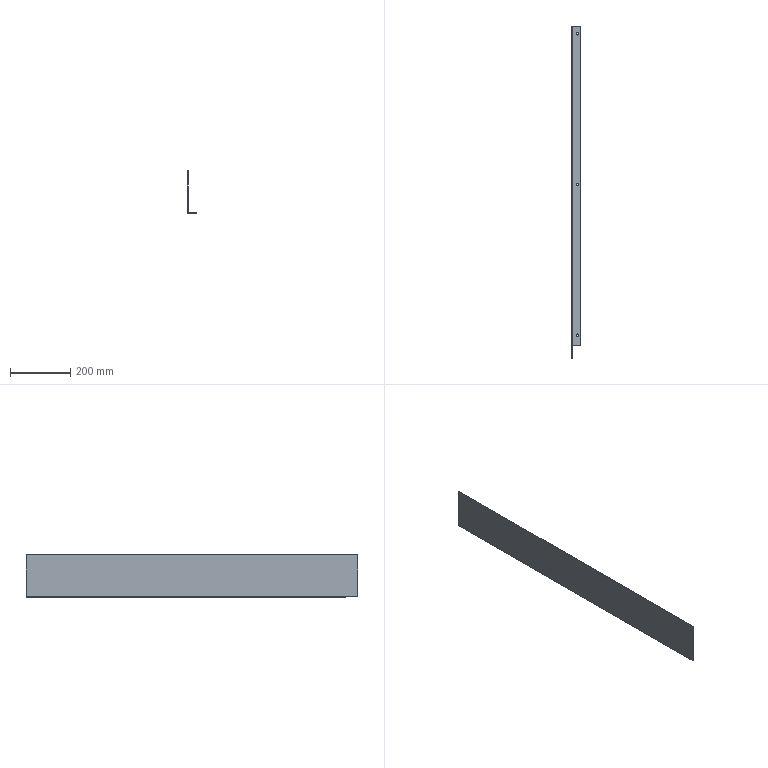Part | STEP file | PN_0008 Partition plate2 | 1 solid | 18 faces | box 30 x 1100 x 140 mm | volume 365122 mm3 | plane 10 | cone 6 | cylinder 2 | commonest cylinder face diameters 2 x1 6 x1
STEP:
#1=CARTESIAN_POINT('',(0.,0.,0.));
#2=DIRECTION('',(0.,0.,1.));
#3=DIRECTION('',(1.,0.,0.));
#4=AXIS2_PLACEMENT_3D('',#1,#2,#3);
#5=CARTESIAN_POINT('',(22.7,525.,0.));
#6=VERTEX_POINT('',#5);
#7=CARTESIAN_POINT('',(24.7,525.,2.));
#8=VERTEX_POINT('',#7);
#9=CARTESIAN_POINT('',(24.7,525.,2.));
#10=DIRECTION('',(0.7071,0.,0.7071));
#11=VECTOR('',#10,1.);
#12=LINE('',#9,#11);
#13=CARTESIAN_POINT('',(20.,525.,2.));
#14=DIRECTION('',(0.,0.,1.));
#15=DIRECTION('',(1.,0.,0.));
#16=AXIS2_PLACEMENT_3D('',#13,#14,#15);
#17=CONICAL_SURFACE('',#16,4.7,0.7854);
#18=CARTESIAN_POINT('',(6.283,0.));
#19=DIRECTION('',(0.,1.));
#20=VECTOR('',#19,1.);
#21=LINE('',#18,#20);
#22=(GEOMETRIC_REPRESENTATION_CONTEXT(2)PARAMETRIC_REPRESENTATION_CONTEXT()REPRESENTATION_CONTEXT('',''));
#23=DEFINITIONAL_REPRESENTATION('',(#21),#22);
#24=PCURVE('',#17,#23);
#25=CARTESIAN_POINT('',(20.,525.,2.));
#26=DIRECTION('',(0.,0.,1.));
#27=DIRECTION('',(1.,0.,0.));
#28=AXIS2_PLACEMENT_3D('',#25,#26,#27);
#29=CONICAL_SURFACE('',#28,4.7,0.7854);
#30=CARTESIAN_POINT('',(0.,0.));
#31=DIRECTION('',(0.,1.));
#32=VECTOR('',#31,1.);
#33=LINE('',#30,#32);
#34=(GEOMETRIC_REPRESENTATION_CONTEXT(2)PARAMETRIC_REPRESENTATION_CONTEXT()REPRESENTATION_CONTEXT('',''));
#35=DEFINITIONAL_REPRESENTATION('',(#33),#34);
#36=PCURVE('',#29,#35);
#37=SURFACE_CURVE('',#12,(#24,#36),.PCURVE_S1.);
#38=EDGE_CURVE('',#6,#8,#37,.T.);
#39=ORIENTED_EDGE('',*,*,#38,.T.);
#40=CARTESIAN_POINT('',(15.3,525.,2.));
#41=VERTEX_POINT('',#40);
#42=CARTESIAN_POINT('',(20.,525.,2.));
#43=DIRECTION('',(0.,0.,1.));
#44=DIRECTION('',(1.,0.,0.));
#45=AXIS2_PLACEMENT_3D('',#42,#43,#44);
#46=CIRCLE('',#45,4.7);
#47=CARTESIAN_POINT('',(0.,0.));
#48=DIRECTION('',(1.,0.));
#49=VECTOR('',#48,1.);
#50=LINE('',#47,#49);
#51=(GEOMETRIC_REPRESENTATION_CONTEXT(2)PARAMETRIC_REPRESENTATION_CONTEXT()REPRESENTATION_CONTEXT('',''));
#52=DEFINITIONAL_REPRESENTATION('',(#50),#51);
#53=PCURVE('',#17,#52);
#54=CARTESIAN_POINT('',(30.,550.,2.));
#55=DIRECTION('',(0.,0.,-1.));
#56=DIRECTION('',(-1.,0.,0.));
#57=AXIS2_PLACEMENT_3D('',#54,#55,#56);
#58=PLANE('',#57);
#59=CARTESIAN_POINT('',(5.3,-25.));
#60=CARTESIAN_POINT('',(5.3,-16.859));
#61=CARTESIAN_POINT('',(12.35,-20.93));
#62=CARTESIAN_POINT('',(19.4,-25.));
#63=CARTESIAN_POINT('',(12.35,-29.07));
#64=CARTESIAN_POINT('',(5.3,-33.141));
#65=CARTESIAN_POINT('',(5.3,-25.));
#66=(BOUNDED_CURVE()B_SPLINE_CURVE(2,(#59,#60,#61,#62,#63,#64,#65),.UNSPECIFIED.,.T.,.F.)B_SPLINE_CURVE_WITH_KNOTS((1,2,2,2,2,1),(-2.094,0.,2.094,4.189,6.283,8.378),.UNSPECIFIED.)CURVE()GEOMETRIC_REPRESENTATION_ITEM()RATIONAL_B_SPLINE_CURVE((1.,0.5,1.,0.5,1.,0.5,1.))REPRESENTATION_ITEM(''));
#67=(GEOMETRIC_REPRESENTATION_CONTEXT(2)PARAMETRIC_REPRESENTATION_CONTEXT()REPRESENTATION_CONTEXT('',''));
#68=DEFINITIONAL_REPRESENTATION('',(#66),#67);
#69=PCURVE('',#58,#68);
#70=SURFACE_CURVE('',#46,(#53,#69),.PCURVE_S1.);
#71=EDGE_CURVE('',#41,#8,#70,.T.);
#72=ORIENTED_EDGE('',*,*,#71,.F.);
#73=CARTESIAN_POINT('',(17.3,525.,0.));
#74=VERTEX_POINT('',#73);
#75=CARTESIAN_POINT('',(15.3,525.,2.));
#76=DIRECTION('',(-0.7071,0.,0.7071));
#77=VECTOR('',#76,1.);
#78=LINE('',#75,#77);
#79=CARTESIAN_POINT('',(3.142,0.));
#80=DIRECTION('',(0.,1.));
#81=VECTOR('',#80,1.);
#82=LINE('',#79,#81);
#83=(GEOMETRIC_REPRESENTATION_CONTEXT(2)PARAMETRIC_REPRESENTATION_CONTEXT()REPRESENTATION_CONTEXT('',''));
#84=DEFINITIONAL_REPRESENTATION('',(#82),#83);
#85=PCURVE('',#17,#84);
#86=CARTESIAN_POINT('',(3.142,0.));
#87=DIRECTION('',(0.,1.));
#88=VECTOR('',#87,1.);
#89=LINE('',#86,#88);
#90=(GEOMETRIC_REPRESENTATION_CONTEXT(2)PARAMETRIC_REPRESENTATION_CONTEXT()REPRESENTATION_CONTEXT('',''));
#91=DEFINITIONAL_REPRESENTATION('',(#89),#90);
#92=PCURVE('',#29,#91);
#93=SURFACE_CURVE('',#78,(#85,#92),.PCURVE_S1.);
#94=EDGE_CURVE('',#74,#41,#93,.T.);
#95=ORIENTED_EDGE('',*,*,#94,.F.);
#96=CARTESIAN_POINT('',(20.,525.,0.));
#97=DIRECTION('',(0.,0.,1.));
#98=DIRECTION('',(1.,0.,0.));
#99=AXIS2_PLACEMENT_3D('',#96,#97,#98);
#100=CIRCLE('',#99,2.7);
#101=CARTESIAN_POINT('',(0.,-2.));
#102=DIRECTION('',(1.,0.));
#103=VECTOR('',#102,1.);
#104=LINE('',#101,#103);
#105=(GEOMETRIC_REPRESENTATION_CONTEXT(2)PARAMETRIC_REPRESENTATION_CONTEXT()REPRESENTATION_CONTEXT('',''));
#106=DEFINITIONAL_REPRESENTATION('',(#104),#105);
#107=PCURVE('',#17,#106);
#108=CARTESIAN_POINT('',(3.,550.,0.));
#109=DIRECTION('',(0.,0.,1.));
#110=DIRECTION('',(1.,0.,0.));
#111=AXIS2_PLACEMENT_3D('',#108,#109,#110);
#112=PLANE('',#111);
#113=CARTESIAN_POINT('',(17.,-25.));
#114=DIRECTION('',(1.,0.));
#115=AXIS2_PLACEMENT_2D('',#113,#114);
#116=CIRCLE('',#115,2.7);
#117=(GEOMETRIC_REPRESENTATION_CONTEXT(2)PARAMETRIC_REPRESENTATION_CONTEXT()REPRESENTATION_CONTEXT('',''));
#118=DEFINITIONAL_REPRESENTATION('',(#116),#117);
#119=PCURVE('',#112,#118);
#120=SURFACE_CURVE('',#100,(#107,#119),.PCURVE_S1.);
#121=EDGE_CURVE('',#74,#6,#120,.T.);
#122=ORIENTED_EDGE('',*,*,#121,.T.);
#123=EDGE_LOOP('',(#39,#72,#95,#122));
#124=FACE_BOUND('',#123,.F.);
#125=ADVANCED_FACE('',(#124),#17,.F.);
#126=CARTESIAN_POINT('',(22.7,25.,0.));
#127=VERTEX_POINT('',#126);
#128=CARTESIAN_POINT('',(24.7,25.,2.));
#129=VERTEX_POINT('',#128);
#130=CARTESIAN_POINT('',(24.7,25.,2.));
#131=DIRECTION('',(0.7071,0.,0.7071));
#132=VECTOR('',#131,1.);
#133=LINE('',#130,#132);
#134=CARTESIAN_POINT('',(20.,25.,2.));
#135=DIRECTION('',(0.,0.,1.));
#136=DIRECTION('',(1.,0.,0.));
#137=AXIS2_PLACEMENT_3D('',#134,#135,#136);
#138=CONICAL_SURFACE('',#137,4.7,0.7854);
#139=CARTESIAN_POINT('',(6.283,0.));
#140=DIRECTION('',(0.,1.));
#141=VECTOR('',#140,1.);
#142=LINE('',#139,#141);
#143=(GEOMETRIC_REPRESENTATION_CONTEXT(2)PARAMETRIC_REPRESENTATION_CONTEXT()REPRESENTATION_CONTEXT('',''));
#144=DEFINITIONAL_REPRESENTATION('',(#142),#143);
#145=PCURVE('',#138,#144);
#146=CARTESIAN_POINT('',(20.,25.,2.));
#147=DIRECTION('',(0.,0.,1.));
#148=DIRECTION('',(1.,0.,0.));
#149=AXIS2_PLACEMENT_3D('',#146,#147,#148);
#150=CONICAL_SURFACE('',#149,4.7,0.7854);
#151=CARTESIAN_POINT('',(0.,0.));
#152=DIRECTION('',(0.,1.));
#153=VECTOR('',#152,1.);
#154=LINE('',#151,#153);
#155=(GEOMETRIC_REPRESENTATION_CONTEXT(2)PARAMETRIC_REPRESENTATION_CONTEXT()REPRESENTATION_CONTEXT('',''));
#156=DEFINITIONAL_REPRESENTATION('',(#154),#155);
#157=PCURVE('',#150,#156);
#158=SURFACE_CURVE('',#133,(#145,#157),.PCURVE_S1.);
#159=EDGE_CURVE('',#127,#129,#158,.T.);
#160=ORIENTED_EDGE('',*,*,#159,.T.);
#161=CARTESIAN_POINT('',(15.3,25.,2.));
#162=VERTEX_POINT('',#161);
#163=CARTESIAN_POINT('',(20.,25.,2.));
#164=DIRECTION('',(0.,0.,1.));
#165=DIRECTION('',(1.,0.,0.));
#166=AXIS2_PLACEMENT_3D('',#163,#164,#165);
#167=CIRCLE('',#166,4.7);
#168=CARTESIAN_POINT('',(0.,0.));
#169=DIRECTION('',(1.,0.));
#170=VECTOR('',#169,1.);
#171=LINE('',#168,#170);
#172=(GEOMETRIC_REPRESENTATION_CONTEXT(2)PARAMETRIC_REPRESENTATION_CONTEXT()REPRESENTATION_CONTEXT('',''));
#173=DEFINITIONAL_REPRESENTATION('',(#171),#172);
#174=PCURVE('',#138,#173);
#175=CARTESIAN_POINT('',(5.3,-525.));
#176=CARTESIAN_POINT('',(5.3,-516.859));
#177=CARTESIAN_POINT('',(12.35,-520.93));
#178=CARTESIAN_POINT('',(19.4,-525.));
#179=CARTESIAN_POINT('',(12.35,-529.07));
#180=CARTESIAN_POINT('',(5.3,-533.141));
#181=CARTESIAN_POINT('',(5.3,-525.));
#182=(BOUNDED_CURVE()B_SPLINE_CURVE(2,(#175,#176,#177,#178,#179,#180,#181),.UNSPECIFIED.,.T.,.F.)B_SPLINE_CURVE_WITH_KNOTS((1,2,2,2,2,1),(-2.094,0.,2.094,4.189,6.283,8.378),.UNSPECIFIED.)CURVE()GEOMETRIC_REPRESENTATION_ITEM()RATIONAL_B_SPLINE_CURVE((1.,0.5,1.,0.5,1.,0.5,1.))REPRESENTATION_ITEM(''));
#183=(GEOMETRIC_REPRESENTATION_CONTEXT(2)PARAMETRIC_REPRESENTATION_CONTEXT()REPRESENTATION_CONTEXT('',''));
#184=DEFINITIONAL_REPRESENTATION('',(#182),#183);
#185=PCURVE('',#58,#184);
#186=SURFACE_CURVE('',#167,(#174,#185),.PCURVE_S1.);
#187=EDGE_CURVE('',#162,#129,#186,.T.);
#188=ORIENTED_EDGE('',*,*,#187,.F.);
#189=CARTESIAN_POINT('',(17.3,25.,0.));
#190=VERTEX_POINT('',#189);
#191=CARTESIAN_POINT('',(15.3,25.,2.));
#192=DIRECTION('',(-0.7071,0.,0.7071));
#193=VECTOR('',#192,1.);
#194=LINE('',#191,#193);
#195=CARTESIAN_POINT('',(3.142,0.));
#196=DIRECTION('',(0.,1.));
#197=VECTOR('',#196,1.);
#198=LINE('',#195,#197);
#199=(GEOMETRIC_REPRESENTATION_CONTEXT(2)PARAMETRIC_REPRESENTATION_CONTEXT()REPRESENTATION_CONTEXT('',''));
#200=DEFINITIONAL_REPRESENTATION('',(#198),#199);
#201=PCURVE('',#138,#200);
#202=CARTESIAN_POINT('',(3.142,0.));
#203=DIRECTION('',(0.,1.));
#204=VECTOR('',#203,1.);
#205=LINE('',#202,#204);
#206=(GEOMETRIC_REPRESENTATION_CONTEXT(2)PARAMETRIC_REPRESENTATION_CONTEXT()REPRESENTATION_CONTEXT('',''));
#207=DEFINITIONAL_REPRESENTATION('',(#205),#206);
#208=PCURVE('',#150,#207);
#209=SURFACE_CURVE('',#194,(#201,#208),.PCURVE_S1.);
#210=EDGE_CURVE('',#190,#162,#209,.T.);
#211=ORIENTED_EDGE('',*,*,#210,.F.);
#212=CARTESIAN_POINT('',(20.,25.,0.));
#213=DIRECTION('',(0.,0.,1.));
#214=DIRECTION('',(1.,0.,0.));
#215=AXIS2_PLACEMENT_3D('',#212,#213,#214);
#216=CIRCLE('',#215,2.7);
#217=CARTESIAN_POINT('',(0.,-2.));
#218=DIRECTION('',(1.,0.));
#219=VECTOR('',#218,1.);
#220=LINE('',#217,#219);
#221=(GEOMETRIC_REPRESENTATION_CONTEXT(2)PARAMETRIC_REPRESENTATION_CONTEXT()REPRESENTATION_CONTEXT('',''));
#222=DEFINITIONAL_REPRESENTATION('',(#220),#221);
#223=PCURVE('',#138,#222);
#224=CARTESIAN_POINT('',(17.,-525.));
#225=DIRECTION('',(1.,0.));
#226=AXIS2_PLACEMENT_2D('',#224,#225);
#227=CIRCLE('',#226,2.7);
#228=(GEOMETRIC_REPRESENTATION_CONTEXT(2)PARAMETRIC_REPRESENTATION_CONTEXT()REPRESENTATION_CONTEXT('',''));
#229=DEFINITIONAL_REPRESENTATION('',(#227),#228);
#230=PCURVE('',#112,#229);
#231=SURFACE_CURVE('',#216,(#223,#230),.PCURVE_S1.);
#232=EDGE_CURVE('',#190,#127,#231,.T.);
#233=ORIENTED_EDGE('',*,*,#232,.T.);
#234=EDGE_LOOP('',(#160,#188,#211,#233));
#235=FACE_BOUND('',#234,.F.);
#236=ADVANCED_FACE('',(#235),#138,.F.);
#237=CARTESIAN_POINT('',(22.7,-475.,0.));
#238=VERTEX_POINT('',#237);
#239=CARTESIAN_POINT('',(24.7,-475.,2.));
#240=VERTEX_POINT('',#239);
#241=CARTESIAN_POINT('',(24.7,-475.,2.));
#242=DIRECTION('',(0.7071,0.,0.7071));
#243=VECTOR('',#242,1.);
#244=LINE('',#241,#243);
#245=CARTESIAN_POINT('',(20.,-475.,2.));
#246=DIRECTION('',(0.,0.,1.));
#247=DIRECTION('',(1.,0.,0.));
#248=AXIS2_PLACEMENT_3D('',#245,#246,#247);
#249=CONICAL_SURFACE('',#248,4.7,0.7854);
#250=CARTESIAN_POINT('',(6.283,0.));
#251=DIRECTION('',(0.,1.));
#252=VECTOR('',#251,1.);
#253=LINE('',#250,#252);
#254=(GEOMETRIC_REPRESENTATION_CONTEXT(2)PARAMETRIC_REPRESENTATION_CONTEXT()REPRESENTATION_CONTEXT('',''));
#255=DEFINITIONAL_REPRESENTATION('',(#253),#254);
#256=PCURVE('',#249,#255);
#257=CARTESIAN_POINT('',(20.,-475.,2.));
#258=DIRECTION('',(0.,0.,1.));
#259=DIRECTION('',(1.,0.,0.));
#260=AXIS2_PLACEMENT_3D('',#257,#258,#259);
#261=CONICAL_SURFACE('',#260,4.7,0.7854);
#262=CARTESIAN_POINT('',(0.,0.));
#263=DIRECTION('',(0.,1.));
#264=VECTOR('',#263,1.);
#265=LINE('',#262,#264);
#266=(GEOMETRIC_REPRESENTATION_CONTEXT(2)PARAMETRIC_REPRESENTATION_CONTEXT()REPRESENTATION_CONTEXT('',''));
#267=DEFINITIONAL_REPRESENTATION('',(#265),#266);
#268=PCURVE('',#261,#267);
#269=SURFACE_CURVE('',#244,(#256,#268),.PCURVE_S1.);
#270=EDGE_CURVE('',#238,#240,#269,.T.);
#271=ORIENTED_EDGE('',*,*,#270,.T.);
#272=CARTESIAN_POINT('',(15.3,-475.,2.));
#273=VERTEX_POINT('',#272);
#274=CARTESIAN_POINT('',(20.,-475.,2.));
#275=DIRECTION('',(0.,0.,1.));
#276=DIRECTION('',(1.,0.,0.));
#277=AXIS2_PLACEMENT_3D('',#274,#275,#276);
#278=CIRCLE('',#277,4.7);
#279=CARTESIAN_POINT('',(0.,0.));
#280=DIRECTION('',(1.,0.));
#281=VECTOR('',#280,1.);
#282=LINE('',#279,#281);
#283=(GEOMETRIC_REPRESENTATION_CONTEXT(2)PARAMETRIC_REPRESENTATION_CONTEXT()REPRESENTATION_CONTEXT('',''));
#284=DEFINITIONAL_REPRESENTATION('',(#282),#283);
#285=PCURVE('',#249,#284);
#286=CARTESIAN_POINT('',(5.3,-1025.));
#287=CARTESIAN_POINT('',(5.3,-1016.859));
#288=CARTESIAN_POINT('',(12.35,-1020.93));
#289=CARTESIAN_POINT('',(19.4,-1025.));
#290=CARTESIAN_POINT('',(12.35,-1029.07));
#291=CARTESIAN_POINT('',(5.3,-1033.141));
#292=CARTESIAN_POINT('',(5.3,-1025.));
#293=(BOUNDED_CURVE()B_SPLINE_CURVE(2,(#286,#287,#288,#289,#290,#291,#292),.UNSPECIFIED.,.T.,.F.)B_SPLINE_CURVE_WITH_KNOTS((1,2,2,2,2,1),(-2.094,0.,2.094,4.189,6.283,8.378),.UNSPECIFIED.)CURVE()GEOMETRIC_REPRESENTATION_ITEM()RATIONAL_B_SPLINE_CURVE((1.,0.5,1.,0.5,1.,0.5,1.))REPRESENTATION_ITEM(''));
#294=(GEOMETRIC_REPRESENTATION_CONTEXT(2)PARAMETRIC_REPRESENTATION_CONTEXT()REPRESENTATION_CONTEXT('',''));
#295=DEFINITIONAL_REPRESENTATION('',(#293),#294);
#296=PCURVE('',#58,#295);
#297=SURFACE_CURVE('',#278,(#285,#296),.PCURVE_S1.);
#298=EDGE_CURVE('',#273,#240,#297,.T.);
#299=ORIENTED_EDGE('',*,*,#298,.F.);
#300=CARTESIAN_POINT('',(17.3,-475.,0.));
#301=VERTEX_POINT('',#300);
#302=CARTESIAN_POINT('',(15.3,-475.,2.));
#303=DIRECTION('',(-0.7071,0.,0.7071));
#304=VECTOR('',#303,1.);
#305=LINE('',#302,#304);
#306=CARTESIAN_POINT('',(3.142,0.));
#307=DIRECTION('',(0.,1.));
#308=VECTOR('',#307,1.);
#309=LINE('',#306,#308);
#310=(GEOMETRIC_REPRESENTATION_CONTEXT(2)PARAMETRIC_REPRESENTATION_CONTEXT()REPRESENTATION_CONTEXT('',''));
#311=DEFINITIONAL_REPRESENTATION('',(#309),#310);
#312=PCURVE('',#249,#311);
#313=CARTESIAN_POINT('',(3.142,0.));
#314=DIRECTION('',(0.,1.));
#315=VECTOR('',#314,1.);
#316=LINE('',#313,#315);
#317=(GEOMETRIC_REPRESENTATION_CONTEXT(2)PARAMETRIC_REPRESENTATION_CONTEXT()REPRESENTATION_CONTEXT('',''));
#318=DEFINITIONAL_REPRESENTATION('',(#316),#317);
#319=PCURVE('',#261,#318);
#320=SURFACE_CURVE('',#305,(#312,#319),.PCURVE_S1.);
#321=EDGE_CURVE('',#301,#273,#320,.T.);
#322=ORIENTED_EDGE('',*,*,#321,.F.);
#323=CARTESIAN_POINT('',(20.,-475.,0.));
#324=DIRECTION('',(0.,0.,1.));
#325=DIRECTION('',(1.,0.,0.));
#326=AXIS2_PLACEMENT_3D('',#323,#324,#325);
#327=CIRCLE('',#326,2.7);
#328=CARTESIAN_POINT('',(0.,-2.));
#329=DIRECTION('',(1.,0.));
#330=VECTOR('',#329,1.);
#331=LINE('',#328,#330);
#332=(GEOMETRIC_REPRESENTATION_CONTEXT(2)PARAMETRIC_REPRESENTATION_CONTEXT()REPRESENTATION_CONTEXT('',''));
#333=DEFINITIONAL_REPRESENTATION('',(#331),#332);
#334=PCURVE('',#249,#333);
#335=CARTESIAN_POINT('',(17.,-1025.));
#336=DIRECTION('',(1.,0.));
#337=AXIS2_PLACEMENT_2D('',#335,#336);
#338=CIRCLE('',#337,2.7);
#339=(GEOMETRIC_REPRESENTATION_CONTEXT(2)PARAMETRIC_REPRESENTATION_CONTEXT()REPRESENTATION_CONTEXT('',''));
#340=DEFINITIONAL_REPRESENTATION('',(#338),#339);
#341=PCURVE('',#112,#340);
#342=SURFACE_CURVE('',#327,(#334,#341),.PCURVE_S1.);
#343=EDGE_CURVE('',#301,#238,#342,.T.);
#344=ORIENTED_EDGE('',*,*,#343,.T.);
#345=EDGE_LOOP('',(#271,#299,#322,#344));
#346=FACE_BOUND('',#345,.F.);
#347=ADVANCED_FACE('',(#346),#249,.F.);
#348=CARTESIAN_POINT('',(20.,525.,2.));
#349=DIRECTION('',(0.,0.,1.));
#350=DIRECTION('',(1.,0.,0.));
#351=AXIS2_PLACEMENT_3D('',#348,#349,#350);
#352=CIRCLE('',#351,4.7);
#353=CARTESIAN_POINT('',(5.3,-25.));
#354=CARTESIAN_POINT('',(5.3,-16.859));
#355=CARTESIAN_POINT('',(12.35,-20.93));
#356=CARTESIAN_POINT('',(19.4,-25.));
#357=CARTESIAN_POINT('',(12.35,-29.07));
#358=CARTESIAN_POINT('',(5.3,-33.141));
#359=CARTESIAN_POINT('',(5.3,-25.));
#360=(BOUNDED_CURVE()B_SPLINE_CURVE(2,(#353,#354,#355,#356,#357,#358,#359),.UNSPECIFIED.,.T.,.F.)B_SPLINE_CURVE_WITH_KNOTS((1,2,2,2,2,1),(-2.094,0.,2.094,4.189,6.283,8.378),.UNSPECIFIED.)CURVE()GEOMETRIC_REPRESENTATION_ITEM()RATIONAL_B_SPLINE_CURVE((1.,0.5,1.,0.5,1.,0.5,1.))REPRESENTATION_ITEM(''));
#361=(GEOMETRIC_REPRESENTATION_CONTEXT(2)PARAMETRIC_REPRESENTATION_CONTEXT()REPRESENTATION_CONTEXT('',''));
#362=DEFINITIONAL_REPRESENTATION('',(#360),#361);
#363=PCURVE('',#58,#362);
#364=CARTESIAN_POINT('',(0.,0.));
#365=DIRECTION('',(1.,0.));
#366=VECTOR('',#365,1.);
#367=LINE('',#364,#366);
#368=(GEOMETRIC_REPRESENTATION_CONTEXT(2)PARAMETRIC_REPRESENTATION_CONTEXT()REPRESENTATION_CONTEXT('',''));
#369=DEFINITIONAL_REPRESENTATION('',(#367),#368);
#370=PCURVE('',#29,#369);
#371=SURFACE_CURVE('',#352,(#363,#370),.PCURVE_S1.);
#372=EDGE_CURVE('',#8,#41,#371,.T.);
#373=ORIENTED_EDGE('',*,*,#372,.F.);
#374=ORIENTED_EDGE('',*,*,#71,.F.);
#375=EDGE_LOOP('',(#373,#374));
#376=FACE_BOUND('',#375,.T.);
#377=CARTESIAN_POINT('',(20.,-475.,2.));
#378=DIRECTION('',(0.,0.,1.));
#379=DIRECTION('',(1.,0.,0.));
#380=AXIS2_PLACEMENT_3D('',#377,#378,#379);
#381=CIRCLE('',#380,4.7);
#382=CARTESIAN_POINT('',(5.3,-1025.));
#383=CARTESIAN_POINT('',(5.3,-1016.859));
#384=CARTESIAN_POINT('',(12.35,-1020.93));
#385=CARTESIAN_POINT('',(19.4,-1025.));
#386=CARTESIAN_POINT('',(12.35,-1029.07));
#387=CARTESIAN_POINT('',(5.3,-1033.141));
#388=CARTESIAN_POINT('',(5.3,-1025.));
#389=(BOUNDED_CURVE()B_SPLINE_CURVE(2,(#382,#383,#384,#385,#386,#387,#388),.UNSPECIFIED.,.T.,.F.)B_SPLINE_CURVE_WITH_KNOTS((1,2,2,2,2,1),(-2.094,0.,2.094,4.189,6.283,8.378),.UNSPECIFIED.)CURVE()GEOMETRIC_REPRESENTATION_ITEM()RATIONAL_B_SPLINE_CURVE((1.,0.5,1.,0.5,1.,0.5,1.))REPRESENTATION_ITEM(''));
#390=(GEOMETRIC_REPRESENTATION_CONTEXT(2)PARAMETRIC_REPRESENTATION_CONTEXT()REPRESENTATION_CONTEXT('',''));
#391=DEFINITIONAL_REPRESENTATION('',(#389),#390);
#392=PCURVE('',#58,#391);
#393=CARTESIAN_POINT('',(0.,0.));
#394=DIRECTION('',(1.,0.));
#395=VECTOR('',#394,1.);
#396=LINE('',#393,#395);
#397=(GEOMETRIC_REPRESENTATION_CONTEXT(2)PARAMETRIC_REPRESENTATION_CONTEXT()REPRESENTATION_CONTEXT('',''));
#398=DEFINITIONAL_REPRESENTATION('',(#396),#397);
#399=PCURVE('',#261,#398);
#400=SURFACE_CURVE('',#381,(#392,#399),.PCURVE_S1.);
#401=EDGE_CURVE('',#240,#273,#400,.T.);
#402=ORIENTED_EDGE('',*,*,#401,.F.);
#403=ORIENTED_EDGE('',*,*,#298,.F.);
#404=EDGE_LOOP('',(#402,#403));
#405=FACE_BOUND('',#404,.T.);
#406=CARTESIAN_POINT('',(3.,550.,2.));
#407=VERTEX_POINT('',#406);
#408=CARTESIAN_POINT('',(3.,-510.,2.));
#409=VERTEX_POINT('',#408);
#410=CARTESIAN_POINT('',(3.,550.,2.));
#411=DIRECTION('',(0.,-1.,0.));
#412=VECTOR('',#411,1.);
#413=LINE('',#410,#412);
#414=CARTESIAN_POINT('',(27.,0.));
#415=DIRECTION('',(0.,-1.));
#416=VECTOR('',#415,1.);
#417=LINE('',#414,#416);
#418=(GEOMETRIC_REPRESENTATION_CONTEXT(2)PARAMETRIC_REPRESENTATION_CONTEXT()REPRESENTATION_CONTEXT('',''));
#419=DEFINITIONAL_REPRESENTATION('',(#417),#418);
#420=PCURVE('',#58,#419);
#421=CARTESIAN_POINT('',(3.,550.,3.));
#422=DIRECTION('',(0.,-1.,0.));
#423=DIRECTION('',(0.,0.,-1.));
#424=AXIS2_PLACEMENT_3D('',#421,#422,#423);
#425=CYLINDRICAL_SURFACE('',#424,1.);
#426=CARTESIAN_POINT('',(6.283,0.));
#427=DIRECTION('',(0.,1.));
#428=VECTOR('',#427,1.);
#429=LINE('',#426,#428);
#430=(GEOMETRIC_REPRESENTATION_CONTEXT(2)PARAMETRIC_REPRESENTATION_CONTEXT()REPRESENTATION_CONTEXT('',''));
#431=DEFINITIONAL_REPRESENTATION('',(#429),#430);
#432=PCURVE('',#425,#431);
#433=SURFACE_CURVE('',#413,(#420,#432),.PCURVE_S1.);
#434=EDGE_CURVE('',#407,#409,#433,.T.);
#435=ORIENTED_EDGE('',*,*,#434,.T.);
#436=CARTESIAN_POINT('',(30.,-510.,2.));
#437=VERTEX_POINT('',#436);
#438=CARTESIAN_POINT('',(30.,-510.,2.));
#439=DIRECTION('',(-1.,0.,0.));
#440=VECTOR('',#439,1.);
#441=LINE('',#438,#440);
#442=CARTESIAN_POINT('',(0.,-1060.));
#443=DIRECTION('',(1.,0.));
#444=VECTOR('',#443,1.);
#445=LINE('',#442,#444);
#446=(GEOMETRIC_REPRESENTATION_CONTEXT(2)PARAMETRIC_REPRESENTATION_CONTEXT()REPRESENTATION_CONTEXT('',''));
#447=DEFINITIONAL_REPRESENTATION('',(#445),#446);
#448=PCURVE('',#58,#447);
#449=CARTESIAN_POINT('',(30.,-510.,0.));
#450=DIRECTION('',(0.,1.,0.));
#451=DIRECTION('',(0.,0.,1.));
#452=AXIS2_PLACEMENT_3D('',#449,#450,#451);
#453=PLANE('',#452);
#454=CARTESIAN_POINT('',(2.,0.));
#455=DIRECTION('',(0.,-1.));
#456=VECTOR('',#455,1.);
#457=LINE('',#454,#456);
#458=(GEOMETRIC_REPRESENTATION_CONTEXT(2)PARAMETRIC_REPRESENTATION_CONTEXT()REPRESENTATION_CONTEXT('',''));
#459=DEFINITIONAL_REPRESENTATION('',(#457),#458);
#460=PCURVE('',#453,#459);
#461=SURFACE_CURVE('',#441,(#448,#460),.PCURVE_S1.);
#462=EDGE_CURVE('',#437,#409,#461,.T.);
#463=ORIENTED_EDGE('',*,*,#462,.F.);
#464=CARTESIAN_POINT('',(30.,550.,2.));
#465=VERTEX_POINT('',#464);
#466=CARTESIAN_POINT('',(30.,550.,2.));
#467=DIRECTION('',(0.,-1.,0.));
#468=VECTOR('',#467,1.);
#469=LINE('',#466,#468);
#470=CARTESIAN_POINT('',(0.,0.));
#471=DIRECTION('',(0.,-1.));
#472=VECTOR('',#471,1.);
#473=LINE('',#470,#472);
#474=(GEOMETRIC_REPRESENTATION_CONTEXT(2)PARAMETRIC_REPRESENTATION_CONTEXT()REPRESENTATION_CONTEXT('',''));
#475=DEFINITIONAL_REPRESENTATION('',(#473),#474);
#476=PCURVE('',#58,#475);
#477=CARTESIAN_POINT('',(30.,550.,0.));
#478=DIRECTION('',(-1.,0.,0.));
#479=DIRECTION('',(0.,0.,1.));
#480=AXIS2_PLACEMENT_3D('',#477,#478,#479);
#481=PLANE('',#480);
#482=CARTESIAN_POINT('',(2.,0.));
#483=DIRECTION('',(0.,-1.));
#484=VECTOR('',#483,1.);
#485=LINE('',#482,#484);
#486=(GEOMETRIC_REPRESENTATION_CONTEXT(2)PARAMETRIC_REPRESENTATION_CONTEXT()REPRESENTATION_CONTEXT('',''));
#487=DEFINITIONAL_REPRESENTATION('',(#485),#486);
#488=PCURVE('',#481,#487);
#489=SURFACE_CURVE('',#469,(#476,#488),.PCURVE_S1.);
#490=EDGE_CURVE('',#465,#437,#489,.T.);
#491=ORIENTED_EDGE('',*,*,#490,.F.);
#492=CARTESIAN_POINT('',(30.,550.,2.));
#493=DIRECTION('',(1.,0.,0.));
#494=VECTOR('',#493,1.);
#495=LINE('',#492,#494);
#496=CARTESIAN_POINT('',(0.,0.));
#497=DIRECTION('',(-1.,0.));
#498=VECTOR('',#497,1.);
#499=LINE('',#496,#498);
#500=(GEOMETRIC_REPRESENTATION_CONTEXT(2)PARAMETRIC_REPRESENTATION_CONTEXT()REPRESENTATION_CONTEXT('',''));
#501=DEFINITIONAL_REPRESENTATION('',(#499),#500);
#502=PCURVE('',#58,#501);
#503=CARTESIAN_POINT('',(3.,550.,3.));
#504=DIRECTION('',(0.,-1.,0.));
#505=DIRECTION('',(0.,0.,-1.));
#506=AXIS2_PLACEMENT_3D('',#503,#504,#505);
#507=PLANE('',#506);
#508=CARTESIAN_POINT('',(1.,27.));
#509=DIRECTION('',(0.,1.));
#510=VECTOR('',#509,1.);
#511=LINE('',#508,#510);
#512=(GEOMETRIC_REPRESENTATION_CONTEXT(2)PARAMETRIC_REPRESENTATION_CONTEXT()REPRESENTATION_CONTEXT('',''));
#513=DEFINITIONAL_REPRESENTATION('',(#511),#512);
#514=PCURVE('',#507,#513);
#515=SURFACE_CURVE('',#495,(#502,#514),.PCURVE_S1.);
#516=EDGE_CURVE('',#407,#465,#515,.T.);
#517=ORIENTED_EDGE('',*,*,#516,.F.);
#518=EDGE_LOOP('',(#435,#463,#491,#517));
#519=FACE_BOUND('',#518,.T.);
#520=CARTESIAN_POINT('',(20.,25.,2.));
#521=DIRECTION('',(0.,0.,1.));
#522=DIRECTION('',(1.,0.,0.));
#523=AXIS2_PLACEMENT_3D('',#520,#521,#522);
#524=CIRCLE('',#523,4.7);
#525=CARTESIAN_POINT('',(5.3,-525.));
#526=CARTESIAN_POINT('',(5.3,-516.859));
#527=CARTESIAN_POINT('',(12.35,-520.93));
#528=CARTESIAN_POINT('',(19.4,-525.));
#529=CARTESIAN_POINT('',(12.35,-529.07));
#530=CARTESIAN_POINT('',(5.3,-533.141));
#531=CARTESIAN_POINT('',(5.3,-525.));
#532=(BOUNDED_CURVE()B_SPLINE_CURVE(2,(#525,#526,#527,#528,#529,#530,#531),.UNSPECIFIED.,.T.,.F.)B_SPLINE_CURVE_WITH_KNOTS((1,2,2,2,2,1),(-2.094,0.,2.094,4.189,6.283,8.378),.UNSPECIFIED.)CURVE()GEOMETRIC_REPRESENTATION_ITEM()RATIONAL_B_SPLINE_CURVE((1.,0.5,1.,0.5,1.,0.5,1.))REPRESENTATION_ITEM(''));
#533=(GEOMETRIC_REPRESENTATION_CONTEXT(2)PARAMETRIC_REPRESENTATION_CONTEXT()REPRESENTATION_CONTEXT('',''));
#534=DEFINITIONAL_REPRESENTATION('',(#532),#533);
#535=PCURVE('',#58,#534);
#536=CARTESIAN_POINT('',(0.,0.));
#537=DIRECTION('',(1.,0.));
#538=VECTOR('',#537,1.);
#539=LINE('',#536,#538);
#540=(GEOMETRIC_REPRESENTATION_CONTEXT(2)PARAMETRIC_REPRESENTATION_CONTEXT()REPRESENTATION_CONTEXT('',''));
#541=DEFINITIONAL_REPRESENTATION('',(#539),#540);
#542=PCURVE('',#150,#541);
#543=SURFACE_CURVE('',#524,(#535,#542),.PCURVE_S1.);
#544=EDGE_CURVE('',#129,#162,#543,.T.);
#545=ORIENTED_EDGE('',*,*,#544,.F.);
#546=ORIENTED_EDGE('',*,*,#187,.F.);
#547=EDGE_LOOP('',(#545,#546));
#548=FACE_BOUND('',#547,.T.);
#549=ADVANCED_FACE('',(#376,#405,#519,#548),#58,.F.);
#550=CARTESIAN_POINT('',(0.,-550.,140.));
#551=VERTEX_POINT('',#550);
#552=CARTESIAN_POINT('',(2.,-550.,140.));
#553=VERTEX_POINT('',#552);
#554=CARTESIAN_POINT('',(2.,-550.,140.));
#555=DIRECTION('',(1.,0.,0.));
#556=VECTOR('',#555,1.);
#557=LINE('',#554,#556);
#558=CARTESIAN_POINT('',(2.,550.,140.));
#559=DIRECTION('',(0.,0.,-1.));
#560=DIRECTION('',(-1.,0.,0.));
#561=AXIS2_PLACEMENT_3D('',#558,#559,#560);
#562=PLANE('',#561);
#563=CARTESIAN_POINT('',(0.,-1100.));
#564=DIRECTION('',(-1.,0.));
#565=VECTOR('',#564,1.);
#566=LINE('',#563,#565);
#567=(GEOMETRIC_REPRESENTATION_CONTEXT(2)PARAMETRIC_REPRESENTATION_CONTEXT()REPRESENTATION_CONTEXT('',''));
#568=DEFINITIONAL_REPRESENTATION('',(#566),#567);
#569=PCURVE('',#562,#568);
#570=CARTESIAN_POINT('',(3.,-550.,3.));
#571=DIRECTION('',(0.,-1.,0.));
#572=DIRECTION('',(0.,0.,-1.));
#573=AXIS2_PLACEMENT_3D('',#570,#571,#572);
#574=PLANE('',#573);
#575=CARTESIAN_POINT('',(-137.,-1.));
#576=DIRECTION('',(0.,1.));
#577=VECTOR('',#576,1.);
#578=LINE('',#575,#577);
#579=(GEOMETRIC_REPRESENTATION_CONTEXT(2)PARAMETRIC_REPRESENTATION_CONTEXT()REPRESENTATION_CONTEXT('',''));
#580=DEFINITIONAL_REPRESENTATION('',(#578),#579);
#581=PCURVE('',#574,#580);
#582=SURFACE_CURVE('',#557,(#569,#581),.PCURVE_S1.);
#583=EDGE_CURVE('',#551,#553,#582,.T.);
#584=ORIENTED_EDGE('',*,*,#583,.T.);
#585=CARTESIAN_POINT('',(2.,550.,140.));
#586=VERTEX_POINT('',#585);
#587=CARTESIAN_POINT('',(2.,550.,140.));
#588=DIRECTION('',(0.,-1.,0.));
#589=VECTOR('',#588,1.);
#590=LINE('',#587,#589);
#591=CARTESIAN_POINT('',(0.,0.));
#592=DIRECTION('',(0.,-1.));
#593=VECTOR('',#592,1.);
#594=LINE('',#591,#593);
#595=(GEOMETRIC_REPRESENTATION_CONTEXT(2)PARAMETRIC_REPRESENTATION_CONTEXT()REPRESENTATION_CONTEXT('',''));
#596=DEFINITIONAL_REPRESENTATION('',(#594),#595);
#597=PCURVE('',#562,#596);
#598=CARTESIAN_POINT('',(2.,550.,3.));
#599=DIRECTION('',(-1.,0.,0.));
#600=DIRECTION('',(0.,0.,1.));
#601=AXIS2_PLACEMENT_3D('',#598,#599,#600);
#602=PLANE('',#601);
#603=CARTESIAN_POINT('',(137.,0.));
#604=DIRECTION('',(0.,-1.));
#605=VECTOR('',#604,1.);
#606=LINE('',#603,#605);
#607=(GEOMETRIC_REPRESENTATION_CONTEXT(2)PARAMETRIC_REPRESENTATION_CONTEXT()REPRESENTATION_CONTEXT('',''));
#608=DEFINITIONAL_REPRESENTATION('',(#606),#607);
#609=PCURVE('',#602,#608);
#610=SURFACE_CURVE('',#590,(#597,#609),.PCURVE_S1.);
#611=EDGE_CURVE('',#586,#553,#610,.T.);
#612=ORIENTED_EDGE('',*,*,#611,.F.);
#613=CARTESIAN_POINT('',(0.,550.,140.));
#614=VERTEX_POINT('',#613);
#615=CARTESIAN_POINT('',(2.,550.,140.));
#616=DIRECTION('',(1.,0.,0.));
#617=VECTOR('',#616,1.);
#618=LINE('',#615,#617);
#619=CARTESIAN_POINT('',(0.,0.));
#620=DIRECTION('',(-1.,0.));
#621=VECTOR('',#620,1.);
#622=LINE('',#619,#621);
#623=(GEOMETRIC_REPRESENTATION_CONTEXT(2)PARAMETRIC_REPRESENTATION_CONTEXT()REPRESENTATION_CONTEXT('',''));
#624=DEFINITIONAL_REPRESENTATION('',(#622),#623);
#625=PCURVE('',#562,#624);
#626=CARTESIAN_POINT('',(-137.,-1.));
#627=DIRECTION('',(0.,1.));
#628=VECTOR('',#627,1.);
#629=LINE('',#626,#628);
#630=(GEOMETRIC_REPRESENTATION_CONTEXT(2)PARAMETRIC_REPRESENTATION_CONTEXT()REPRESENTATION_CONTEXT('',''));
#631=DEFINITIONAL_REPRESENTATION('',(#629),#630);
#632=PCURVE('',#507,#631);
#633=SURFACE_CURVE('',#618,(#625,#632),.PCURVE_S1.);
#634=EDGE_CURVE('',#614,#586,#633,.T.);
#635=ORIENTED_EDGE('',*,*,#634,.F.);
#636=CARTESIAN_POINT('',(0.,550.,140.));
#637=DIRECTION('',(0.,-1.,0.));
#638=VECTOR('',#637,1.);
#639=LINE('',#636,#638);
#640=CARTESIAN_POINT('',(2.,0.));
#641=DIRECTION('',(0.,-1.));
#642=VECTOR('',#641,1.);
#643=LINE('',#640,#642);
#644=(GEOMETRIC_REPRESENTATION_CONTEXT(2)PARAMETRIC_REPRESENTATION_CONTEXT()REPRESENTATION_CONTEXT('',''));
#645=DEFINITIONAL_REPRESENTATION('',(#643),#644);
#646=PCURVE('',#562,#645);
#647=CARTESIAN_POINT('',(0.,550.,140.));
#648=DIRECTION('',(1.,0.,0.));
#649=DIRECTION('',(0.,0.,-1.));
#650=AXIS2_PLACEMENT_3D('',#647,#648,#649);
#651=PLANE('',#650);
#652=CARTESIAN_POINT('',(0.,0.));
#653=DIRECTION('',(0.,-1.));
#654=VECTOR('',#653,1.);
#655=LINE('',#652,#654);
#656=(GEOMETRIC_REPRESENTATION_CONTEXT(2)PARAMETRIC_REPRESENTATION_CONTEXT()REPRESENTATION_CONTEXT('',''));
#657=DEFINITIONAL_REPRESENTATION('',(#655),#656);
#658=PCURVE('',#651,#657);
#659=SURFACE_CURVE('',#639,(#646,#658),.PCURVE_S1.);
#660=EDGE_CURVE('',#614,#551,#659,.T.);
#661=ORIENTED_EDGE('',*,*,#660,.T.);
#662=EDGE_LOOP('',(#584,#612,#635,#661));
#663=FACE_BOUND('',#662,.T.);
#664=ADVANCED_FACE('',(#663),#562,.F.);
#665=CARTESIAN_POINT('',(2.,-550.,3.));
#666=VERTEX_POINT('',#665);
#667=CARTESIAN_POINT('',(2.,-550.,3.));
#668=DIRECTION('',(0.,0.,-1.));
#669=VECTOR('',#668,1.);
#670=LINE('',#667,#669);
#671=CARTESIAN_POINT('',(0.,-1100.));
#672=DIRECTION('',(-1.,0.));
#673=VECTOR('',#672,1.);
#674=LINE('',#671,#673);
#675=(GEOMETRIC_REPRESENTATION_CONTEXT(2)PARAMETRIC_REPRESENTATION_CONTEXT()REPRESENTATION_CONTEXT('',''));
#676=DEFINITIONAL_REPRESENTATION('',(#674),#675);
#677=PCURVE('',#602,#676);
#678=CARTESIAN_POINT('',(0.,-1.));
#679=DIRECTION('',(1.,0.));
#680=VECTOR('',#679,1.);
#681=LINE('',#678,#680);
#682=(GEOMETRIC_REPRESENTATION_CONTEXT(2)PARAMETRIC_REPRESENTATION_CONTEXT()REPRESENTATION_CONTEXT('',''));
#683=DEFINITIONAL_REPRESENTATION('',(#681),#682);
#684=PCURVE('',#574,#683);
#685=SURFACE_CURVE('',#670,(#677,#684),.PCURVE_S1.);
#686=EDGE_CURVE('',#553,#666,#685,.T.);
#687=ORIENTED_EDGE('',*,*,#686,.T.);
#688=CARTESIAN_POINT('',(2.,550.,3.));
#689=VERTEX_POINT('',#688);
#690=CARTESIAN_POINT('',(2.,550.,3.));
#691=DIRECTION('',(0.,-1.,0.));
#692=VECTOR('',#691,1.);
#693=LINE('',#690,#692);
#694=CARTESIAN_POINT('',(0.,0.));
#695=DIRECTION('',(0.,-1.));
#696=VECTOR('',#695,1.);
#697=LINE('',#694,#696);
#698=(GEOMETRIC_REPRESENTATION_CONTEXT(2)PARAMETRIC_REPRESENTATION_CONTEXT()REPRESENTATION_CONTEXT('',''));
#699=DEFINITIONAL_REPRESENTATION('',(#697),#698);
#700=PCURVE('',#602,#699);
#701=CARTESIAN_POINT('',(4.712,0.));
#702=DIRECTION('',(0.,1.));
#703=VECTOR('',#702,1.);
#704=LINE('',#701,#703);
#705=(GEOMETRIC_REPRESENTATION_CONTEXT(2)PARAMETRIC_REPRESENTATION_CONTEXT()REPRESENTATION_CONTEXT('',''));
#706=DEFINITIONAL_REPRESENTATION('',(#704),#705);
#707=PCURVE('',#425,#706);
#708=SURFACE_CURVE('',#693,(#700,#707),.PCURVE_S1.);
#709=EDGE_CURVE('',#689,#666,#708,.T.);
#710=ORIENTED_EDGE('',*,*,#709,.F.);
#711=CARTESIAN_POINT('',(2.,550.,3.));
#712=DIRECTION('',(0.,0.,-1.));
#713=VECTOR('',#712,1.);
#714=LINE('',#711,#713);
#715=CARTESIAN_POINT('',(0.,0.));
#716=DIRECTION('',(-1.,0.));
#717=VECTOR('',#716,1.);
#718=LINE('',#715,#717);
#719=(GEOMETRIC_REPRESENTATION_CONTEXT(2)PARAMETRIC_REPRESENTATION_CONTEXT()REPRESENTATION_CONTEXT('',''));
#720=DEFINITIONAL_REPRESENTATION('',(#718),#719);
#721=PCURVE('',#602,#720);
#722=CARTESIAN_POINT('',(0.,-1.));
#723=DIRECTION('',(1.,0.));
#724=VECTOR('',#723,1.);
#725=LINE('',#722,#724);
#726=(GEOMETRIC_REPRESENTATION_CONTEXT(2)PARAMETRIC_REPRESENTATION_CONTEXT()REPRESENTATION_CONTEXT('',''));
#727=DEFINITIONAL_REPRESENTATION('',(#725),#726);
#728=PCURVE('',#507,#727);
#729=SURFACE_CURVE('',#714,(#721,#728),.PCURVE_S1.);
#730=EDGE_CURVE('',#586,#689,#729,.T.);
#731=ORIENTED_EDGE('',*,*,#730,.F.);
#732=ORIENTED_EDGE('',*,*,#611,.T.);
#733=EDGE_LOOP('',(#687,#710,#731,#732));
#734=FACE_BOUND('',#733,.T.);
#735=ADVANCED_FACE('',(#734),#602,.F.);
#736=ORIENTED_EDGE('',*,*,#709,.F.);
#737=CARTESIAN_POINT('',(3.,550.,3.));
#738=DIRECTION('',(0.,-1.,0.));
#739=DIRECTION('',(0.,0.,-1.));
#740=AXIS2_PLACEMENT_3D('',#737,#738,#739);
#741=CIRCLE('',#740,1.);
#742=CARTESIAN_POINT('',(0.,0.));
#743=DIRECTION('',(1.,0.));
#744=VECTOR('',#743,1.);
#745=LINE('',#742,#744);
#746=(GEOMETRIC_REPRESENTATION_CONTEXT(2)PARAMETRIC_REPRESENTATION_CONTEXT()REPRESENTATION_CONTEXT('',''));
#747=DEFINITIONAL_REPRESENTATION('',(#745),#746);
#748=PCURVE('',#425,#747);
#749=CARTESIAN_POINT('',(0.,0.));
#750=DIRECTION('',(1.,0.));
#751=AXIS2_PLACEMENT_2D('',#749,#750);
#752=CIRCLE('',#751,1.);
#753=(GEOMETRIC_REPRESENTATION_CONTEXT(2)PARAMETRIC_REPRESENTATION_CONTEXT()REPRESENTATION_CONTEXT('',''));
#754=DEFINITIONAL_REPRESENTATION('',(#752),#753);
#755=PCURVE('',#507,#754);
#756=SURFACE_CURVE('',#741,(#748,#755),.PCURVE_S1.);
#757=EDGE_CURVE('',#689,#407,#756,.T.);
#758=ORIENTED_EDGE('',*,*,#757,.T.);
#759=ORIENTED_EDGE('',*,*,#434,.T.);
#760=CARTESIAN_POINT('',(3.,-550.,2.));
#761=VERTEX_POINT('',#760);
#762=CARTESIAN_POINT('',(3.,550.,2.));
#763=DIRECTION('',(0.,1.,0.));
#764=VECTOR('',#763,1.);
#765=LINE('',#762,#764);
#766=CARTESIAN_POINT('',(6.283,0.));
#767=DIRECTION('',(0.,-1.));
#768=VECTOR('',#767,1.);
#769=LINE('',#766,#768);
#770=(GEOMETRIC_REPRESENTATION_CONTEXT(2)PARAMETRIC_REPRESENTATION_CONTEXT()REPRESENTATION_CONTEXT('',''));
#771=DEFINITIONAL_REPRESENTATION('',(#769),#770);
#772=PCURVE('',#425,#771);
#773=CARTESIAN_POINT('',(0.,0.,2.));
#774=DIRECTION('',(0.,0.,1.));
#775=DIRECTION('',(1.,0.,0.));
#776=AXIS2_PLACEMENT_3D('',#773,#774,#775);
#777=PLANE('',#776);
#778=CARTESIAN_POINT('',(3.,550.));
#779=DIRECTION('',(0.,1.));
#780=VECTOR('',#779,1.);
#781=LINE('',#778,#780);
#782=(GEOMETRIC_REPRESENTATION_CONTEXT(2)PARAMETRIC_REPRESENTATION_CONTEXT()REPRESENTATION_CONTEXT('',''));
#783=DEFINITIONAL_REPRESENTATION('',(#781),#782);
#784=PCURVE('',#777,#783);
#785=SURFACE_CURVE('',#765,(#772,#784),.PCURVE_S1.);
#786=EDGE_CURVE('',#761,#409,#785,.T.);
#787=ORIENTED_EDGE('',*,*,#786,.F.);
#788=CARTESIAN_POINT('',(3.,-550.,3.));
#789=DIRECTION('',(0.,-1.,0.));
#790=DIRECTION('',(0.,0.,-1.));
#791=AXIS2_PLACEMENT_3D('',#788,#789,#790);
#792=CIRCLE('',#791,1.);
#793=CARTESIAN_POINT('',(0.,1100.));
#794=DIRECTION('',(1.,0.));
#795=VECTOR('',#794,1.);
#796=LINE('',#793,#795);
#797=(GEOMETRIC_REPRESENTATION_CONTEXT(2)PARAMETRIC_REPRESENTATION_CONTEXT()REPRESENTATION_CONTEXT('',''));
#798=DEFINITIONAL_REPRESENTATION('',(#796),#797);
#799=PCURVE('',#425,#798);
#800=CARTESIAN_POINT('',(0.,0.));
#801=DIRECTION('',(1.,0.));
#802=AXIS2_PLACEMENT_2D('',#800,#801);
#803=CIRCLE('',#802,1.);
#804=(GEOMETRIC_REPRESENTATION_CONTEXT(2)PARAMETRIC_REPRESENTATION_CONTEXT()REPRESENTATION_CONTEXT('',''));
#805=DEFINITIONAL_REPRESENTATION('',(#803),#804);
#806=PCURVE('',#574,#805);
#807=SURFACE_CURVE('',#792,(#799,#806),.PCURVE_S1.);
#808=EDGE_CURVE('',#666,#761,#807,.T.);
#809=ORIENTED_EDGE('',*,*,#808,.F.);
#810=EDGE_LOOP('',(#736,#758,#759,#787,#809));
#811=FACE_BOUND('',#810,.F.);
#812=ADVANCED_FACE('',(#811),#425,.F.);
#813=ORIENTED_EDGE('',*,*,#490,.T.);
#814=CARTESIAN_POINT('',(30.,-510.,0.));
#815=VERTEX_POINT('',#814);
#816=CARTESIAN_POINT('',(30.,-510.,0.));
#817=DIRECTION('',(0.,0.,1.));
#818=VECTOR('',#817,1.);
#819=LINE('',#816,#818);
#820=CARTESIAN_POINT('',(0.,-1060.));
#821=DIRECTION('',(1.,0.));
#822=VECTOR('',#821,1.);
#823=LINE('',#820,#822);
#824=(GEOMETRIC_REPRESENTATION_CONTEXT(2)PARAMETRIC_REPRESENTATION_CONTEXT()REPRESENTATION_CONTEXT('',''));
#825=DEFINITIONAL_REPRESENTATION('',(#823),#824);
#826=PCURVE('',#481,#825);
#827=CARTESIAN_POINT('',(0.,0.));
#828=DIRECTION('',(1.,0.));
#829=VECTOR('',#828,1.);
#830=LINE('',#827,#829);
#831=(GEOMETRIC_REPRESENTATION_CONTEXT(2)PARAMETRIC_REPRESENTATION_CONTEXT()REPRESENTATION_CONTEXT('',''));
#832=DEFINITIONAL_REPRESENTATION('',(#830),#831);
#833=PCURVE('',#453,#832);
#834=SURFACE_CURVE('',#819,(#826,#833),.PCURVE_S1.);
#835=EDGE_CURVE('',#815,#437,#834,.T.);
#836=ORIENTED_EDGE('',*,*,#835,.F.);
#837=CARTESIAN_POINT('',(30.,550.,0.));
#838=VERTEX_POINT('',#837);
#839=CARTESIAN_POINT('',(30.,550.,0.));
#840=DIRECTION('',(0.,-1.,0.));
#841=VECTOR('',#840,1.);
#842=LINE('',#839,#841);
#843=CARTESIAN_POINT('',(0.,0.));
#844=DIRECTION('',(0.,-1.));
#845=VECTOR('',#844,1.);
#846=LINE('',#843,#845);
#847=(GEOMETRIC_REPRESENTATION_CONTEXT(2)PARAMETRIC_REPRESENTATION_CONTEXT()REPRESENTATION_CONTEXT('',''));
#848=DEFINITIONAL_REPRESENTATION('',(#846),#847);
#849=PCURVE('',#481,#848);
#850=CARTESIAN_POINT('',(27.,0.));
#851=DIRECTION('',(0.,-1.));
#852=VECTOR('',#851,1.);
#853=LINE('',#850,#852);
#854=(GEOMETRIC_REPRESENTATION_CONTEXT(2)PARAMETRIC_REPRESENTATION_CONTEXT()REPRESENTATION_CONTEXT('',''));
#855=DEFINITIONAL_REPRESENTATION('',(#853),#854);
#856=PCURVE('',#112,#855);
#857=SURFACE_CURVE('',#842,(#849,#856),.PCURVE_S1.);
#858=EDGE_CURVE('',#838,#815,#857,.T.);
#859=ORIENTED_EDGE('',*,*,#858,.F.);
#860=CARTESIAN_POINT('',(30.,550.,0.));
#861=DIRECTION('',(0.,0.,-1.));
#862=VECTOR('',#861,1.);
#863=LINE('',#860,#862);
#864=CARTESIAN_POINT('',(0.,0.));
#865=DIRECTION('',(-1.,0.));
#866=VECTOR('',#865,1.);
#867=LINE('',#864,#866);
#868=(GEOMETRIC_REPRESENTATION_CONTEXT(2)PARAMETRIC_REPRESENTATION_CONTEXT()REPRESENTATION_CONTEXT('',''));
#869=DEFINITIONAL_REPRESENTATION('',(#867),#868);
#870=PCURVE('',#481,#869);
#871=CARTESIAN_POINT('',(3.,27.));
#872=DIRECTION('',(1.,0.));
#873=VECTOR('',#872,1.);
#874=LINE('',#871,#873);
#875=(GEOMETRIC_REPRESENTATION_CONTEXT(2)PARAMETRIC_REPRESENTATION_CONTEXT()REPRESENTATION_CONTEXT('',''));
#876=DEFINITIONAL_REPRESENTATION('',(#874),#875);
#877=PCURVE('',#507,#876);
#878=SURFACE_CURVE('',#863,(#870,#877),.PCURVE_S1.);
#879=EDGE_CURVE('',#465,#838,#878,.T.);
#880=ORIENTED_EDGE('',*,*,#879,.F.);
#881=EDGE_LOOP('',(#813,#836,#859,#880));
#882=FACE_BOUND('',#881,.T.);
#883=ADVANCED_FACE('',(#882),#481,.F.);
#884=CARTESIAN_POINT('',(20.,525.,0.));
#885=DIRECTION('',(0.,0.,1.));
#886=DIRECTION('',(1.,0.,0.));
#887=AXIS2_PLACEMENT_3D('',#884,#885,#886);
#888=CIRCLE('',#887,2.7);
#889=CARTESIAN_POINT('',(17.,-25.));
#890=DIRECTION('',(1.,0.));
#891=AXIS2_PLACEMENT_2D('',#889,#890);
#892=CIRCLE('',#891,2.7);
#893=(GEOMETRIC_REPRESENTATION_CONTEXT(2)PARAMETRIC_REPRESENTATION_CONTEXT()REPRESENTATION_CONTEXT('',''));
#894=DEFINITIONAL_REPRESENTATION('',(#892),#893);
#895=PCURVE('',#112,#894);
#896=CARTESIAN_POINT('',(0.,-2.));
#897=DIRECTION('',(1.,0.));
#898=VECTOR('',#897,1.);
#899=LINE('',#896,#898);
#900=(GEOMETRIC_REPRESENTATION_CONTEXT(2)PARAMETRIC_REPRESENTATION_CONTEXT()REPRESENTATION_CONTEXT('',''));
#901=DEFINITIONAL_REPRESENTATION('',(#899),#900);
#902=PCURVE('',#29,#901);
#903=SURFACE_CURVE('',#888,(#895,#902),.PCURVE_S1.);
#904=EDGE_CURVE('',#6,#74,#903,.T.);
#905=ORIENTED_EDGE('',*,*,#904,.T.);
#906=ORIENTED_EDGE('',*,*,#121,.T.);
#907=EDGE_LOOP('',(#905,#906));
#908=FACE_BOUND('',#907,.T.);
#909=CARTESIAN_POINT('',(20.,25.,0.));
#910=DIRECTION('',(0.,0.,1.));
#911=DIRECTION('',(1.,0.,0.));
#912=AXIS2_PLACEMENT_3D('',#909,#910,#911);
#913=CIRCLE('',#912,2.7);
#914=CARTESIAN_POINT('',(17.,-525.));
#915=DIRECTION('',(1.,0.));
#916=AXIS2_PLACEMENT_2D('',#914,#915);
#917=CIRCLE('',#916,2.7);
#918=(GEOMETRIC_REPRESENTATION_CONTEXT(2)PARAMETRIC_REPRESENTATION_CONTEXT()REPRESENTATION_CONTEXT('',''));
#919=DEFINITIONAL_REPRESENTATION('',(#917),#918);
#920=PCURVE('',#112,#919);
#921=CARTESIAN_POINT('',(0.,-2.));
#922=DIRECTION('',(1.,0.));
#923=VECTOR('',#922,1.);
#924=LINE('',#921,#923);
#925=(GEOMETRIC_REPRESENTATION_CONTEXT(2)PARAMETRIC_REPRESENTATION_CONTEXT()REPRESENTATION_CONTEXT('',''));
#926=DEFINITIONAL_REPRESENTATION('',(#924),#925);
#927=PCURVE('',#150,#926);
#928=SURFACE_CURVE('',#913,(#920,#927),.PCURVE_S1.);
#929=EDGE_CURVE('',#127,#190,#928,.T.);
#930=ORIENTED_EDGE('',*,*,#929,.T.);
#931=ORIENTED_EDGE('',*,*,#232,.T.);
#932=EDGE_LOOP('',(#930,#931));
#933=FACE_BOUND('',#932,.T.);
#934=CARTESIAN_POINT('',(20.,-475.,0.));
#935=DIRECTION('',(0.,0.,1.));
#936=DIRECTION('',(1.,0.,0.));
#937=AXIS2_PLACEMENT_3D('',#934,#935,#936);
#938=CIRCLE('',#937,2.7);
#939=CARTESIAN_POINT('',(17.,-1025.));
#940=DIRECTION('',(1.,0.));
#941=AXIS2_PLACEMENT_2D('',#939,#940);
#942=CIRCLE('',#941,2.7);
#943=(GEOMETRIC_REPRESENTATION_CONTEXT(2)PARAMETRIC_REPRESENTATION_CONTEXT()REPRESENTATION_CONTEXT('',''));
#944=DEFINITIONAL_REPRESENTATION('',(#942),#943);
#945=PCURVE('',#112,#944);
#946=CARTESIAN_POINT('',(0.,-2.));
#947=DIRECTION('',(1.,0.));
#948=VECTOR('',#947,1.);
#949=LINE('',#946,#948);
#950=(GEOMETRIC_REPRESENTATION_CONTEXT(2)PARAMETRIC_REPRESENTATION_CONTEXT()REPRESENTATION_CONTEXT('',''));
#951=DEFINITIONAL_REPRESENTATION('',(#949),#950);
#952=PCURVE('',#261,#951);
#953=SURFACE_CURVE('',#938,(#945,#952),.PCURVE_S1.);
#954=EDGE_CURVE('',#238,#301,#953,.T.);
#955=ORIENTED_EDGE('',*,*,#954,.T.);
#956=ORIENTED_EDGE('',*,*,#343,.T.);
#957=EDGE_LOOP('',(#955,#956));
#958=FACE_BOUND('',#957,.T.);
#959=ORIENTED_EDGE('',*,*,#858,.T.);
#960=CARTESIAN_POINT('',(3.,-510.,0.));
#961=VERTEX_POINT('',#960);
#962=CARTESIAN_POINT('',(30.,-510.,0.));
#963=DIRECTION('',(-1.,0.,0.));
#964=VECTOR('',#963,1.);
#965=LINE('',#962,#964);
#966=CARTESIAN_POINT('',(27.,-1060.));
#967=DIRECTION('',(-1.,0.));
#968=VECTOR('',#967,1.);
#969=LINE('',#966,#968);
#970=(GEOMETRIC_REPRESENTATION_CONTEXT(2)PARAMETRIC_REPRESENTATION_CONTEXT()REPRESENTATION_CONTEXT('',''));
#971=DEFINITIONAL_REPRESENTATION('',(#969),#970);
#972=PCURVE('',#112,#971);
#973=CARTESIAN_POINT('',(0.,0.));
#974=DIRECTION('',(0.,-1.));
#975=VECTOR('',#974,1.);
#976=LINE('',#973,#975);
#977=(GEOMETRIC_REPRESENTATION_CONTEXT(2)PARAMETRIC_REPRESENTATION_CONTEXT()REPRESENTATION_CONTEXT('',''));
#978=DEFINITIONAL_REPRESENTATION('',(#976),#977);
#979=PCURVE('',#453,#978);
#980=SURFACE_CURVE('',#965,(#972,#979),.PCURVE_S1.);
#981=EDGE_CURVE('',#815,#961,#980,.T.);
#982=ORIENTED_EDGE('',*,*,#981,.T.);
#983=CARTESIAN_POINT('',(3.,550.,0.));
#984=VERTEX_POINT('',#983);
#985=CARTESIAN_POINT('',(3.,550.,0.));
#986=DIRECTION('',(0.,-1.,0.));
#987=VECTOR('',#986,1.);
#988=LINE('',#985,#987);
#989=CARTESIAN_POINT('',(0.,0.));
#990=DIRECTION('',(0.,-1.));
#991=VECTOR('',#990,1.);
#992=LINE('',#989,#991);
#993=(GEOMETRIC_REPRESENTATION_CONTEXT(2)PARAMETRIC_REPRESENTATION_CONTEXT()REPRESENTATION_CONTEXT('',''));
#994=DEFINITIONAL_REPRESENTATION('',(#992),#993);
#995=PCURVE('',#112,#994);
#996=CARTESIAN_POINT('',(3.,550.,3.));
#997=DIRECTION('',(0.,-1.,0.));
#998=DIRECTION('',(0.,0.,-1.));
#999=AXIS2_PLACEMENT_3D('',#996,#997,#998);
#1000=CYLINDRICAL_SURFACE('',#999,3.);
#1001=CARTESIAN_POINT('',(6.283,0.));
#1002=DIRECTION('',(0.,1.));
#1003=VECTOR('',#1002,1.);
#1004=LINE('',#1001,#1003);
#1005=(GEOMETRIC_REPRESENTATION_CONTEXT(2)PARAMETRIC_REPRESENTATION_CONTEXT()REPRESENTATION_CONTEXT('',''));
#1006=DEFINITIONAL_REPRESENTATION('',(#1004),#1005);
#1007=PCURVE('',#1000,#1006);
#1008=SURFACE_CURVE('',#988,(#995,#1007),.PCURVE_S1.);
#1009=EDGE_CURVE('',#984,#961,#1008,.T.);
#1010=ORIENTED_EDGE('',*,*,#1009,.F.);
#1011=CARTESIAN_POINT('',(3.,550.,0.));
#1012=DIRECTION('',(-1.,0.,0.));
#1013=VECTOR('',#1012,1.);
#1014=LINE('',#1011,#1013);
#1015=CARTESIAN_POINT('',(0.,0.));
#1016=DIRECTION('',(-1.,0.));
#1017=VECTOR('',#1016,1.);
#1018=LINE('',#1015,#1017);
#1019=(GEOMETRIC_REPRESENTATION_CONTEXT(2)PARAMETRIC_REPRESENTATION_CONTEXT()REPRESENTATION_CONTEXT('',''));
#1020=DEFINITIONAL_REPRESENTATION('',(#1018),#1019);
#1021=PCURVE('',#112,#1020);
#1022=CARTESIAN_POINT('',(3.,0.));
#1023=DIRECTION('',(0.,-1.));
#1024=VECTOR('',#1023,1.);
#1025=LINE('',#1022,#1024);
#1026=(GEOMETRIC_REPRESENTATION_CONTEXT(2)PARAMETRIC_REPRESENTATION_CONTEXT()REPRESENTATION_CONTEXT('',''));
#1027=DEFINITIONAL_REPRESENTATION('',(#1025),#1026);
#1028=PCURVE('',#507,#1027);
#1029=SURFACE_CURVE('',#1014,(#1021,#1028),.PCURVE_S1.);
#1030=EDGE_CURVE('',#838,#984,#1029,.T.);
#1031=ORIENTED_EDGE('',*,*,#1030,.F.);
#1032=EDGE_LOOP('',(#959,#982,#1010,#1031));
#1033=FACE_BOUND('',#1032,.T.);
#1034=ADVANCED_FACE('',(#908,#933,#958,#1033),#112,.F.);
#1035=ORIENTED_EDGE('',*,*,#1009,.T.);
#1036=CARTESIAN_POINT('',(0.1716,-510.,2.));
#1037=VERTEX_POINT('',#1036);
#1038=CARTESIAN_POINT('',(3.,-510.,3.));
#1039=DIRECTION('',(0.,1.,0.));
#1040=DIRECTION('',(0.,0.,1.));
#1041=AXIS2_PLACEMENT_3D('',#1038,#1039,#1040);
#1042=CIRCLE('',#1041,3.);
#1043=CARTESIAN_POINT('',(9.425,1060.));
#1044=DIRECTION('',(-1.,0.));
#1045=VECTOR('',#1044,1.);
#1046=LINE('',#1043,#1045);
#1047=(GEOMETRIC_REPRESENTATION_CONTEXT(2)PARAMETRIC_REPRESENTATION_CONTEXT()REPRESENTATION_CONTEXT('',''));
#1048=DEFINITIONAL_REPRESENTATION('',(#1046),#1047);
#1049=PCURVE('',#1000,#1048);
#1050=CARTESIAN_POINT('',(3.,-27.));
#1051=DIRECTION('',(1.,0.));
#1052=AXIS2_PLACEMENT_2D('',#1050,#1051);
#1053=CIRCLE('',#1052,3.);
#1054=(GEOMETRIC_REPRESENTATION_CONTEXT(2)PARAMETRIC_REPRESENTATION_CONTEXT()REPRESENTATION_CONTEXT('',''));
#1055=DEFINITIONAL_REPRESENTATION('',(#1053),#1054);
#1056=PCURVE('',#453,#1055);
#1057=SURFACE_CURVE('',#1042,(#1049,#1056),.PCURVE_S1.);
#1058=EDGE_CURVE('',#961,#1037,#1057,.T.);
#1059=ORIENTED_EDGE('',*,*,#1058,.T.);
#1060=CARTESIAN_POINT('',(0.1716,-550.,2.));
#1061=VERTEX_POINT('',#1060);
#1062=CARTESIAN_POINT('',(0.1716,550.,2.));
#1063=DIRECTION('',(0.,-1.,0.));
#1064=VECTOR('',#1063,1.);
#1065=LINE('',#1062,#1064);
#1066=CARTESIAN_POINT('',(5.052,0.));
#1067=DIRECTION('',(0.,1.));
#1068=VECTOR('',#1067,1.);
#1069=LINE('',#1066,#1068);
#1070=(GEOMETRIC_REPRESENTATION_CONTEXT(2)PARAMETRIC_REPRESENTATION_CONTEXT()REPRESENTATION_CONTEXT('',''));
#1071=DEFINITIONAL_REPRESENTATION('',(#1069),#1070);
#1072=PCURVE('',#1000,#1071);
#1073=CARTESIAN_POINT('',(0.1716,550.));
#1074=DIRECTION('',(0.,-1.));
#1075=VECTOR('',#1074,1.);
#1076=LINE('',#1073,#1075);
#1077=(GEOMETRIC_REPRESENTATION_CONTEXT(2)PARAMETRIC_REPRESENTATION_CONTEXT()REPRESENTATION_CONTEXT('',''));
#1078=DEFINITIONAL_REPRESENTATION('',(#1076),#1077);
#1079=PCURVE('',#777,#1078);
#1080=SURFACE_CURVE('',#1065,(#1072,#1079),.PCURVE_S1.);
#1081=EDGE_CURVE('',#1037,#1061,#1080,.T.);
#1082=ORIENTED_EDGE('',*,*,#1081,.T.);
#1083=CARTESIAN_POINT('',(0.,-550.,3.));
#1084=VERTEX_POINT('',#1083);
#1085=CARTESIAN_POINT('',(3.,-550.,3.));
#1086=DIRECTION('',(0.,1.,0.));
#1087=DIRECTION('',(0.,0.,-1.));
#1088=AXIS2_PLACEMENT_3D('',#1085,#1086,#1087);
#1089=CIRCLE('',#1088,3.);
#1090=CARTESIAN_POINT('',(6.283,1100.));
#1091=DIRECTION('',(-1.,0.));
#1092=VECTOR('',#1091,1.);
#1093=LINE('',#1090,#1092);
#1094=(GEOMETRIC_REPRESENTATION_CONTEXT(2)PARAMETRIC_REPRESENTATION_CONTEXT()REPRESENTATION_CONTEXT('',''));
#1095=DEFINITIONAL_REPRESENTATION('',(#1093),#1094);
#1096=PCURVE('',#1000,#1095);
#1097=CARTESIAN_POINT('',(3.,0.));
#1098=CARTESIAN_POINT('',(3.,-5.196));
#1099=CARTESIAN_POINT('',(-1.5,-2.598));
#1100=CARTESIAN_POINT('',(-6.,0.));
#1101=CARTESIAN_POINT('',(-1.5,2.598));
#1102=CARTESIAN_POINT('',(3.,5.196));
#1103=CARTESIAN_POINT('',(3.,0.));
#1104=(BOUNDED_CURVE()B_SPLINE_CURVE(2,(#1097,#1098,#1099,#1100,#1101,#1102,#1103),.UNSPECIFIED.,.T.,.F.)B_SPLINE_CURVE_WITH_KNOTS((1,2,2,2,2,1),(-2.094,0.,2.094,4.189,6.283,8.378),.UNSPECIFIED.)CURVE()GEOMETRIC_REPRESENTATION_ITEM()RATIONAL_B_SPLINE_CURVE((1.,0.5,1.,0.5,1.,0.5,1.))REPRESENTATION_ITEM(''));
#1105=(GEOMETRIC_REPRESENTATION_CONTEXT(2)PARAMETRIC_REPRESENTATION_CONTEXT()REPRESENTATION_CONTEXT('',''));
#1106=DEFINITIONAL_REPRESENTATION('',(#1104),#1105);
#1107=PCURVE('',#574,#1106);
#1108=SURFACE_CURVE('',#1089,(#1096,#1107),.PCURVE_S1.);
#1109=EDGE_CURVE('',#1061,#1084,#1108,.T.);
#1110=ORIENTED_EDGE('',*,*,#1109,.T.);
#1111=CARTESIAN_POINT('',(0.,550.,3.));
#1112=VERTEX_POINT('',#1111);
#1113=CARTESIAN_POINT('',(0.,550.,3.));
#1114=DIRECTION('',(0.,-1.,0.));
#1115=VECTOR('',#1114,1.);
#1116=LINE('',#1113,#1115);
#1117=CARTESIAN_POINT('',(4.712,0.));
#1118=DIRECTION('',(0.,1.));
#1119=VECTOR('',#1118,1.);
#1120=LINE('',#1117,#1119);
#1121=(GEOMETRIC_REPRESENTATION_CONTEXT(2)PARAMETRIC_REPRESENTATION_CONTEXT()REPRESENTATION_CONTEXT('',''));
#1122=DEFINITIONAL_REPRESENTATION('',(#1120),#1121);
#1123=PCURVE('',#1000,#1122);
#1124=CARTESIAN_POINT('',(137.,0.));
#1125=DIRECTION('',(0.,-1.));
#1126=VECTOR('',#1125,1.);
#1127=LINE('',#1124,#1126);
#1128=(GEOMETRIC_REPRESENTATION_CONTEXT(2)PARAMETRIC_REPRESENTATION_CONTEXT()REPRESENTATION_CONTEXT('',''));
#1129=DEFINITIONAL_REPRESENTATION('',(#1127),#1128);
#1130=PCURVE('',#651,#1129);
#1131=SURFACE_CURVE('',#1116,(#1123,#1130),.PCURVE_S1.);
#1132=EDGE_CURVE('',#1112,#1084,#1131,.T.);
#1133=ORIENTED_EDGE('',*,*,#1132,.F.);
#1134=CARTESIAN_POINT('',(3.,550.,3.));
#1135=DIRECTION('',(0.,1.,0.));
#1136=DIRECTION('',(0.,0.,-1.));
#1137=AXIS2_PLACEMENT_3D('',#1134,#1135,#1136);
#1138=CIRCLE('',#1137,3.);
#1139=CARTESIAN_POINT('',(6.283,0.));
#1140=DIRECTION('',(-1.,0.));
#1141=VECTOR('',#1140,1.);
#1142=LINE('',#1139,#1141);
#1143=(GEOMETRIC_REPRESENTATION_CONTEXT(2)PARAMETRIC_REPRESENTATION_CONTEXT()REPRESENTATION_CONTEXT('',''));
#1144=DEFINITIONAL_REPRESENTATION('',(#1142),#1143);
#1145=PCURVE('',#1000,#1144);
#1146=CARTESIAN_POINT('',(3.,0.));
#1147=CARTESIAN_POINT('',(3.,-5.196));
#1148=CARTESIAN_POINT('',(-1.5,-2.598));
#1149=CARTESIAN_POINT('',(-6.,0.));
#1150=CARTESIAN_POINT('',(-1.5,2.598));
#1151=CARTESIAN_POINT('',(3.,5.196));
#1152=CARTESIAN_POINT('',(3.,0.));
#1153=(BOUNDED_CURVE()B_SPLINE_CURVE(2,(#1146,#1147,#1148,#1149,#1150,#1151,#1152),.UNSPECIFIED.,.T.,.F.)B_SPLINE_CURVE_WITH_KNOTS((1,2,2,2,2,1),(-2.094,0.,2.094,4.189,6.283,8.378),.UNSPECIFIED.)CURVE()GEOMETRIC_REPRESENTATION_ITEM()RATIONAL_B_SPLINE_CURVE((1.,0.5,1.,0.5,1.,0.5,1.))REPRESENTATION_ITEM(''));
#1154=(GEOMETRIC_REPRESENTATION_CONTEXT(2)PARAMETRIC_REPRESENTATION_CONTEXT()REPRESENTATION_CONTEXT('',''));
#1155=DEFINITIONAL_REPRESENTATION('',(#1153),#1154);
#1156=PCURVE('',#507,#1155);
#1157=SURFACE_CURVE('',#1138,(#1145,#1156),.PCURVE_S1.);
#1158=EDGE_CURVE('',#984,#1112,#1157,.T.);
#1159=ORIENTED_EDGE('',*,*,#1158,.F.);
#1160=EDGE_LOOP('',(#1035,#1059,#1082,#1110,#1133,#1159));
#1161=FACE_BOUND('',#1160,.T.);
#1162=ADVANCED_FACE('',(#1161),#1000,.T.);
#1163=CARTESIAN_POINT('',(0.,-550.,140.));
#1164=DIRECTION('',(0.,0.,1.));
#1165=VECTOR('',#1164,1.);
#1166=LINE('',#1163,#1165);
#1167=CARTESIAN_POINT('',(0.,-1100.));
#1168=DIRECTION('',(-1.,0.));
#1169=VECTOR('',#1168,1.);
#1170=LINE('',#1167,#1169);
#1171=(GEOMETRIC_REPRESENTATION_CONTEXT(2)PARAMETRIC_REPRESENTATION_CONTEXT()REPRESENTATION_CONTEXT('',''));
#1172=DEFINITIONAL_REPRESENTATION('',(#1170),#1171);
#1173=PCURVE('',#651,#1172);
#1174=CARTESIAN_POINT('',(-137.,-3.));
#1175=DIRECTION('',(-1.,0.));
#1176=VECTOR('',#1175,1.);
#1177=LINE('',#1174,#1176);
#1178=(GEOMETRIC_REPRESENTATION_CONTEXT(2)PARAMETRIC_REPRESENTATION_CONTEXT()REPRESENTATION_CONTEXT('',''));
#1179=DEFINITIONAL_REPRESENTATION('',(#1177),#1178);
#1180=PCURVE('',#574,#1179);
#1181=SURFACE_CURVE('',#1166,(#1173,#1180),.PCURVE_S1.);
#1182=EDGE_CURVE('',#1084,#551,#1181,.T.);
#1183=ORIENTED_EDGE('',*,*,#1182,.T.);
#1184=ORIENTED_EDGE('',*,*,#660,.F.);
#1185=CARTESIAN_POINT('',(0.,550.,140.));
#1186=DIRECTION('',(0.,0.,1.));
#1187=VECTOR('',#1186,1.);
#1188=LINE('',#1185,#1187);
#1189=CARTESIAN_POINT('',(0.,0.));
#1190=DIRECTION('',(-1.,0.));
#1191=VECTOR('',#1190,1.);
#1192=LINE('',#1189,#1191);
#1193=(GEOMETRIC_REPRESENTATION_CONTEXT(2)PARAMETRIC_REPRESENTATION_CONTEXT()REPRESENTATION_CONTEXT('',''));
#1194=DEFINITIONAL_REPRESENTATION('',(#1192),#1193);
#1195=PCURVE('',#651,#1194);
#1196=CARTESIAN_POINT('',(-137.,-3.));
#1197=DIRECTION('',(-1.,0.));
#1198=VECTOR('',#1197,1.);
#1199=LINE('',#1196,#1198);
#1200=(GEOMETRIC_REPRESENTATION_CONTEXT(2)PARAMETRIC_REPRESENTATION_CONTEXT()REPRESENTATION_CONTEXT('',''));
#1201=DEFINITIONAL_REPRESENTATION('',(#1199),#1200);
#1202=PCURVE('',#507,#1201);
#1203=SURFACE_CURVE('',#1188,(#1195,#1202),.PCURVE_S1.);
#1204=EDGE_CURVE('',#1112,#614,#1203,.T.);
#1205=ORIENTED_EDGE('',*,*,#1204,.F.);
#1206=ORIENTED_EDGE('',*,*,#1132,.T.);
#1207=EDGE_LOOP('',(#1183,#1184,#1205,#1206));
#1208=FACE_BOUND('',#1207,.T.);
#1209=ADVANCED_FACE('',(#1208),#651,.F.);
#1210=ORIENTED_EDGE('',*,*,#634,.T.);
#1211=ORIENTED_EDGE('',*,*,#730,.T.);
#1212=ORIENTED_EDGE('',*,*,#757,.T.);
#1213=ORIENTED_EDGE('',*,*,#516,.T.);
#1214=ORIENTED_EDGE('',*,*,#879,.T.);
#1215=ORIENTED_EDGE('',*,*,#1030,.T.);
#1216=ORIENTED_EDGE('',*,*,#1158,.T.);
#1217=ORIENTED_EDGE('',*,*,#1204,.T.);
#1218=EDGE_LOOP('',(#1210,#1211,#1212,#1213,#1214,#1215,#1216,#1217));
#1219=FACE_BOUND('',#1218,.T.);
#1220=ADVANCED_FACE('',(#1219),#507,.F.);
#1221=CARTESIAN_POINT('',(3.,-550.,2.));
#1222=DIRECTION('',(-1.,0.,0.));
#1223=VECTOR('',#1222,1.);
#1224=LINE('',#1221,#1223);
#1225=CARTESIAN_POINT('',(1.,0.));
#1226=DIRECTION('',(0.,-1.));
#1227=VECTOR('',#1226,1.);
#1228=LINE('',#1225,#1227);
#1229=(GEOMETRIC_REPRESENTATION_CONTEXT(2)PARAMETRIC_REPRESENTATION_CONTEXT()REPRESENTATION_CONTEXT('',''));
#1230=DEFINITIONAL_REPRESENTATION('',(#1228),#1229);
#1231=PCURVE('',#574,#1230);
#1232=CARTESIAN_POINT('',(3.,-550.));
#1233=DIRECTION('',(-1.,0.));
#1234=VECTOR('',#1233,1.);
#1235=LINE('',#1232,#1234);
#1236=(GEOMETRIC_REPRESENTATION_CONTEXT(2)PARAMETRIC_REPRESENTATION_CONTEXT()REPRESENTATION_CONTEXT('',''));
#1237=DEFINITIONAL_REPRESENTATION('',(#1235),#1236);
#1238=PCURVE('',#777,#1237);
#1239=SURFACE_CURVE('',#1224,(#1231,#1238),.PCURVE_S1.);
#1240=EDGE_CURVE('',#761,#1061,#1239,.T.);
#1241=ORIENTED_EDGE('',*,*,#1240,.F.);
#1242=ORIENTED_EDGE('',*,*,#808,.F.);
#1243=ORIENTED_EDGE('',*,*,#686,.F.);
#1244=ORIENTED_EDGE('',*,*,#583,.F.);
#1245=ORIENTED_EDGE('',*,*,#1182,.F.);
#1246=ORIENTED_EDGE('',*,*,#1109,.F.);
#1247=EDGE_LOOP('',(#1241,#1242,#1243,#1244,#1245,#1246));
#1248=FACE_BOUND('',#1247,.T.);
#1249=ADVANCED_FACE('',(#1248),#574,.T.);
#1250=ORIENTED_EDGE('',*,*,#401,.F.);
#1251=ORIENTED_EDGE('',*,*,#270,.F.);
#1252=ORIENTED_EDGE('',*,*,#954,.T.);
#1253=ORIENTED_EDGE('',*,*,#321,.T.);
#1254=EDGE_LOOP('',(#1250,#1251,#1252,#1253));
#1255=FACE_BOUND('',#1254,.F.);
#1256=ADVANCED_FACE('',(#1255),#261,.F.);
#1257=ORIENTED_EDGE('',*,*,#544,.F.);
#1258=ORIENTED_EDGE('',*,*,#159,.F.);
#1259=ORIENTED_EDGE('',*,*,#929,.T.);
#1260=ORIENTED_EDGE('',*,*,#210,.T.);
#1261=EDGE_LOOP('',(#1257,#1258,#1259,#1260));
#1262=FACE_BOUND('',#1261,.F.);
#1263=ADVANCED_FACE('',(#1262),#150,.F.);
#1264=ORIENTED_EDGE('',*,*,#372,.F.);
#1265=ORIENTED_EDGE('',*,*,#38,.F.);
#1266=ORIENTED_EDGE('',*,*,#904,.T.);
#1267=ORIENTED_EDGE('',*,*,#94,.T.);
#1268=EDGE_LOOP('',(#1264,#1265,#1266,#1267));
#1269=FACE_BOUND('',#1268,.F.);
#1270=ADVANCED_FACE('',(#1269),#29,.F.);
#1271=ORIENTED_EDGE('',*,*,#981,.F.);
#1272=ORIENTED_EDGE('',*,*,#835,.T.);
#1273=ORIENTED_EDGE('',*,*,#462,.T.);
#1274=CARTESIAN_POINT('',(30.,-510.,2.));
#1275=DIRECTION('',(-1.,0.,0.));
#1276=VECTOR('',#1275,1.);
#1277=LINE('',#1274,#1276);
#1278=CARTESIAN_POINT('',(2.,0.));
#1279=DIRECTION('',(0.,-1.));
#1280=VECTOR('',#1279,1.);
#1281=LINE('',#1278,#1280);
#1282=(GEOMETRIC_REPRESENTATION_CONTEXT(2)PARAMETRIC_REPRESENTATION_CONTEXT()REPRESENTATION_CONTEXT('',''));
#1283=DEFINITIONAL_REPRESENTATION('',(#1281),#1282);
#1284=PCURVE('',#453,#1283);
#1285=CARTESIAN_POINT('',(30.,-510.));
#1286=DIRECTION('',(-1.,0.));
#1287=VECTOR('',#1286,1.);
#1288=LINE('',#1285,#1287);
#1289=(GEOMETRIC_REPRESENTATION_CONTEXT(2)PARAMETRIC_REPRESENTATION_CONTEXT()REPRESENTATION_CONTEXT('',''));
#1290=DEFINITIONAL_REPRESENTATION('',(#1288),#1289);
#1291=PCURVE('',#777,#1290);
#1292=SURFACE_CURVE('',#1277,(#1284,#1291),.PCURVE_S1.);
#1293=EDGE_CURVE('',#409,#1037,#1292,.T.);
#1294=ORIENTED_EDGE('',*,*,#1293,.T.);
#1295=ORIENTED_EDGE('',*,*,#1058,.F.);
#1296=EDGE_LOOP('',(#1271,#1272,#1273,#1294,#1295));
#1297=FACE_BOUND('',#1296,.T.);
#1298=ADVANCED_FACE('',(#1297),#453,.F.);
#1299=ORIENTED_EDGE('',*,*,#1240,.T.);
#1300=ORIENTED_EDGE('',*,*,#1081,.F.);
#1301=ORIENTED_EDGE('',*,*,#1293,.F.);
#1302=ORIENTED_EDGE('',*,*,#786,.F.);
#1303=EDGE_LOOP('',(#1299,#1300,#1301,#1302));
#1304=FACE_BOUND('',#1303,.T.);
#1305=ADVANCED_FACE('',(#1304),#777,.F.);
#1306=CLOSED_SHELL('',(#125,#236,#347,#549,#664,#735,#812,#883,#1034,#1162,#1209,#1220,#1249,#1256,#1263,#1270,#1298,#1305));
#1307=MANIFOLD_SOLID_BREP('',#1306);
#1308=(LENGTH_UNIT()NAMED_UNIT(*)SI_UNIT(.MILLI.,.METRE.));
#1309=UNCERTAINTY_MEASURE_WITH_UNIT(LENGTH_MEASURE(0.0000001),#1308,'','');
#1310=(NAMED_UNIT(*)PLANE_ANGLE_UNIT()SI_UNIT($,.RADIAN.));
#1311=(NAMED_UNIT(*)SI_UNIT($,.STERADIAN.)SOLID_ANGLE_UNIT());
#1312=(GEOMETRIC_REPRESENTATION_CONTEXT(3)GLOBAL_UNCERTAINTY_ASSIGNED_CONTEXT((#1309))GLOBAL_UNIT_ASSIGNED_CONTEXT((#1308,#1310,#1311))REPRESENTATION_CONTEXT('',''));
#1313=ADVANCED_BREP_SHAPE_REPRESENTATION('',(#4,#1307),#1312);